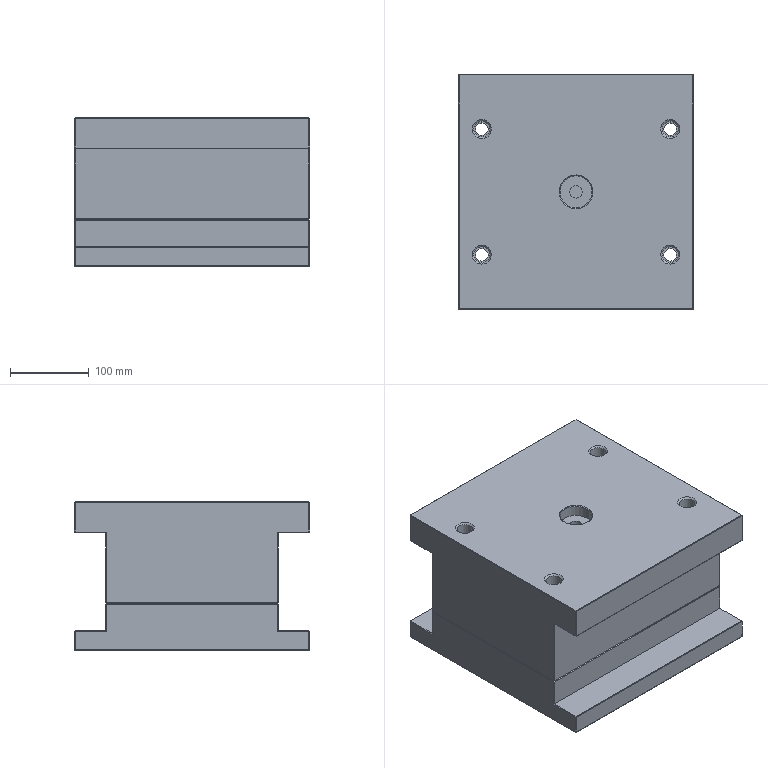NC program | NX | posted with a generic post | part box 300 x 300 x 190 mm
Lines 1803 to 1853 of 1853:
(PLANAR_MILL_COPY_3 , TOOL : D6A45)
N3598 T07 M6
N3600 G17 G43 G0 G90 X-110. Y-80.866 Z30. S7500 H7 M3
N3602 Z0.
N3604 G94 G1 Z-1.5 F1250.
N3606 G3 X-109.5 Y-80. R1.
N3608 X-120. Y-69.5 R10.5
N3610 X-109.5 Y-80. R-10.5
N3612 X-110. Y-79.134 R1.
N3614 G1 Z0.
N3616 G0 Z30.
N3618 Y79.134
N3620 Z0.
N3622 G1 Z-1.5
N3624 G3 X-109.5 Y80. R1.
N3626 X-120. Y90.5 R10.5
N3628 X-109.5 Y80. R-10.5
N3630 X-110. Y80.866 R1.
N3632 G1 Z0.
N3634 G0 Z30.
N3636 X19.5 Y-0.866
N3638 Z0.
N3640 G1 Z-1.5
N3642 G3 X20. Y0. R1.
N3644 X0. Y20. R20.
N3646 X20. Y0. R-20.
N3648 X19.5 Y0.866 R1.
N3650 G1 Z0.
N3652 G0 Z30.
N3654 X130. Y-80.866
N3656 Z0.
N3658 G1 Z-1.5
N3660 G3 X130.5 Y-80. R1.
N3662 X120. Y-69.5 R10.5
N3664 X130.5 Y-80. R-10.5
N3666 X130. Y-79.134 R1.
N3668 G1 Z0.
N3670 G0 Z30.
N3672 Y79.134
N3674 Z0.
N3676 G1 Z-1.5
N3678 G3 X130.5 Y80. R1.
N3680 X120. Y90.5 R10.5
N3682 X130.5 Y80. R-10.5
N3684 X130. Y80.866 R1.
N3686 G1 Z0.
N3688 G0 Z30.
N3690 M5
N3692 M2